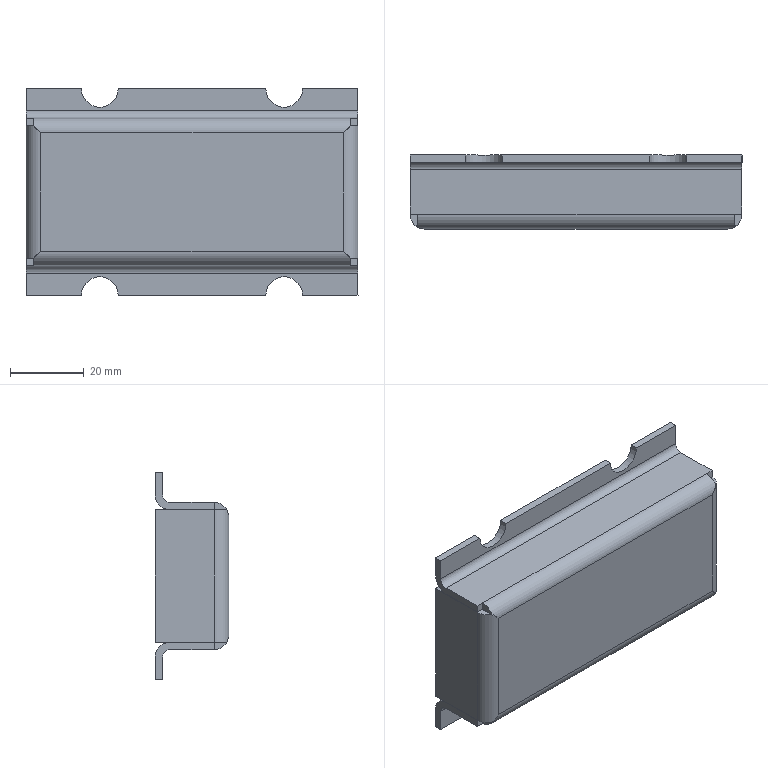Part | NX | features solid 2 | 1 solid | 62 faces | box 90 x 20 x 56 mm | volume 17662 mm3 | plane 46 | cylinder 16 | commonest cylinder face diameters 4 x6 8 x6 10 x4